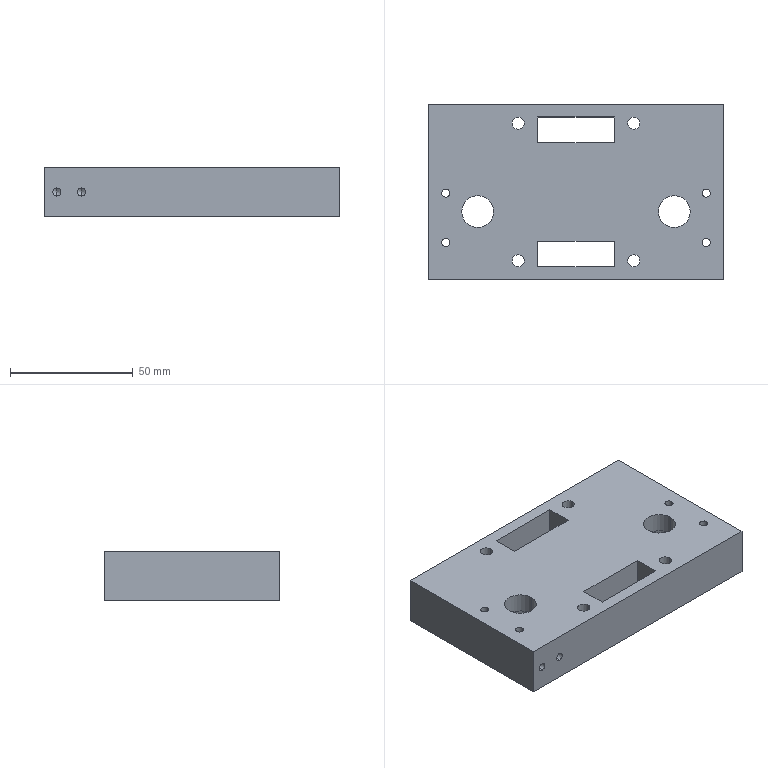Part | 1 solid | 55 faces | box 120 x 71 x 20 mm | volume 135872 mm3 | cylinder 32 | plane 15 | cone 8 | commonest cylinder face diameters 3.3 x16 5 x8 13 x4 19 x4